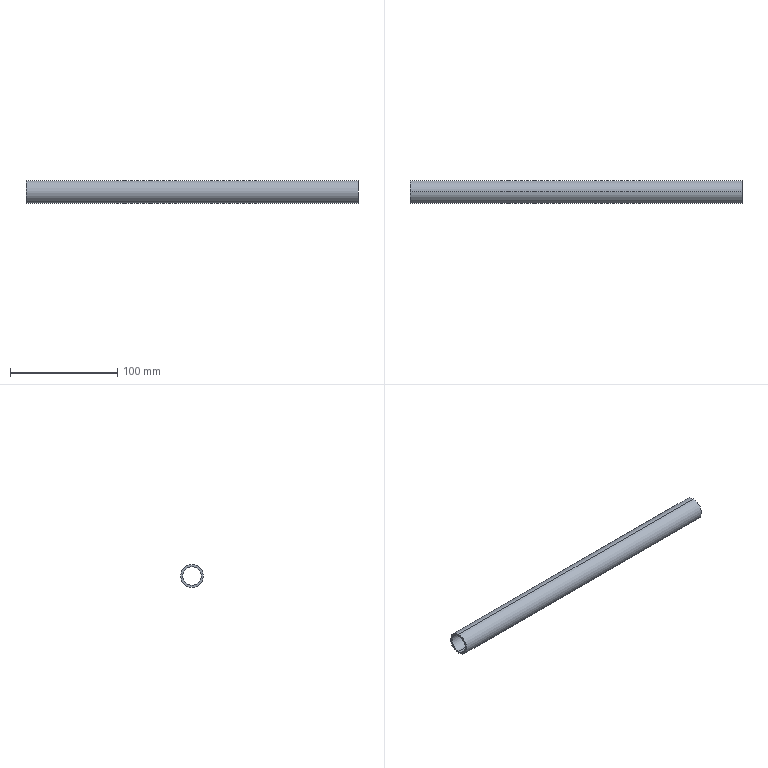Part | SolidWorks | features WeldMemberFeat 1, WeldmentFeature 1 | 1 solid | 6 faces | box 310 x 21.3 x 21.3 mm | volume 37592 mm3 | cylinder 4 | plane 2 | commonest cylinder face diameters 17.3 x2 21.3 x2
STEP:
#1=CARTESIAN_POINT('',(155.,0.,-10.65));
#2=VERTEX_POINT('',#1);
#3=CARTESIAN_POINT('',(155.,0.,10.65));
#4=VERTEX_POINT('',#3);
#5=CARTESIAN_POINT('',(155.,0.,0.));
#6=DIRECTION('',(1.,0.,0.));
#7=DIRECTION('',(0.,0.,-1.));
#8=AXIS2_PLACEMENT_3D('',#5,#6,#7);
#9=CIRCLE('',#8,10.65);
#10=EDGE_CURVE('',#2,#4,#9,.T.);
#11=ORIENTED_EDGE('',*,*,#10,.F.);
#12=CARTESIAN_POINT('',(-155.,0.,-10.65));
#13=VERTEX_POINT('',#12);
#14=CARTESIAN_POINT('',(155.,0.,-10.65));
#15=DIRECTION('',(-1.,0.,0.));
#16=VECTOR('',#15,1000.);
#17=LINE('',#14,#16);
#18=EDGE_CURVE('',#2,#13,#17,.T.);
#19=ORIENTED_EDGE('',*,*,#18,.T.);
#20=CARTESIAN_POINT('',(-155.,0.,10.65));
#21=VERTEX_POINT('',#20);
#22=CARTESIAN_POINT('',(-155.,0.,0.));
#23=DIRECTION('',(1.,0.,0.));
#24=DIRECTION('',(0.,0.,-1.));
#25=AXIS2_PLACEMENT_3D('',#22,#23,#24);
#26=CIRCLE('',#25,10.65);
#27=EDGE_CURVE('',#13,#21,#26,.T.);
#28=ORIENTED_EDGE('',*,*,#27,.T.);
#29=CARTESIAN_POINT('',(155.,0.,10.65));
#30=DIRECTION('',(-1.,0.,0.));
#31=VECTOR('',#30,1000.);
#32=LINE('',#29,#31);
#33=EDGE_CURVE('',#4,#21,#32,.T.);
#34=ORIENTED_EDGE('',*,*,#33,.F.);
#35=EDGE_LOOP('',(#11,#19,#28,#34));
#36=FACE_OUTER_BOUND('',#35,.T.);
#37=CARTESIAN_POINT('',(155.,0.,0.));
#38=DIRECTION('',(-1.,0.,0.));
#39=DIRECTION('',(0.,0.,1.));
#40=AXIS2_PLACEMENT_3D('',#37,#38,#39);
#41=CYLINDRICAL_SURFACE('',#40,10.65);
#42=ADVANCED_FACE('',(#36),#41,.T.);
#43=CARTESIAN_POINT('',(155.,0.,8.65));
#44=VERTEX_POINT('',#43);
#45=CARTESIAN_POINT('',(155.,0.,-8.65));
#46=VERTEX_POINT('',#45);
#47=CARTESIAN_POINT('',(155.,0.,0.));
#48=DIRECTION('',(1.,0.,0.));
#49=DIRECTION('',(0.,0.,-1.));
#50=AXIS2_PLACEMENT_3D('',#47,#48,#49);
#51=CIRCLE('',#50,8.65);
#52=EDGE_CURVE('',#44,#46,#51,.T.);
#53=ORIENTED_EDGE('',*,*,#52,.T.);
#54=CARTESIAN_POINT('',(-155.,0.,-8.65));
#55=VERTEX_POINT('',#54);
#56=CARTESIAN_POINT('',(155.,0.,-8.65));
#57=DIRECTION('',(-1.,0.,0.));
#58=VECTOR('',#57,1000.);
#59=LINE('',#56,#58);
#60=EDGE_CURVE('',#46,#55,#59,.T.);
#61=ORIENTED_EDGE('',*,*,#60,.T.);
#62=CARTESIAN_POINT('',(-155.,0.,8.65));
#63=VERTEX_POINT('',#62);
#64=CARTESIAN_POINT('',(-155.,0.,0.));
#65=DIRECTION('',(1.,0.,0.));
#66=DIRECTION('',(0.,0.,-1.));
#67=AXIS2_PLACEMENT_3D('',#64,#65,#66);
#68=CIRCLE('',#67,8.65);
#69=EDGE_CURVE('',#63,#55,#68,.T.);
#70=ORIENTED_EDGE('',*,*,#69,.F.);
#71=CARTESIAN_POINT('',(155.,0.,8.65));
#72=DIRECTION('',(-1.,0.,0.));
#73=VECTOR('',#72,1000.);
#74=LINE('',#71,#73);
#75=EDGE_CURVE('',#44,#63,#74,.T.);
#76=ORIENTED_EDGE('',*,*,#75,.F.);
#77=EDGE_LOOP('',(#53,#61,#70,#76));
#78=FACE_OUTER_BOUND('',#77,.T.);
#79=CARTESIAN_POINT('',(155.,0.,0.));
#80=DIRECTION('',(-1.,0.,0.));
#81=DIRECTION('',(0.,0.,1.));
#82=AXIS2_PLACEMENT_3D('',#79,#80,#81);
#83=CYLINDRICAL_SURFACE('',#82,8.65);
#84=ADVANCED_FACE('',(#78),#83,.F.);
#85=ORIENTED_EDGE('',*,*,#60,.F.);
#86=CARTESIAN_POINT('',(155.,0.,0.));
#87=DIRECTION('',(1.,0.,0.));
#88=DIRECTION('',(0.,0.,-1.));
#89=AXIS2_PLACEMENT_3D('',#86,#87,#88);
#90=CIRCLE('',#89,8.65);
#91=EDGE_CURVE('',#46,#44,#90,.T.);
#92=ORIENTED_EDGE('',*,*,#91,.T.);
#93=ORIENTED_EDGE('',*,*,#75,.T.);
#94=CARTESIAN_POINT('',(-155.,0.,0.));
#95=DIRECTION('',(1.,0.,0.));
#96=DIRECTION('',(0.,0.,-1.));
#97=AXIS2_PLACEMENT_3D('',#94,#95,#96);
#98=CIRCLE('',#97,8.65);
#99=EDGE_CURVE('',#55,#63,#98,.T.);
#100=ORIENTED_EDGE('',*,*,#99,.F.);
#101=EDGE_LOOP('',(#85,#92,#93,#100));
#102=FACE_OUTER_BOUND('',#101,.T.);
#103=CARTESIAN_POINT('',(155.,0.,0.));
#104=DIRECTION('',(-1.,0.,0.));
#105=DIRECTION('',(0.,0.,1.));
#106=AXIS2_PLACEMENT_3D('',#103,#104,#105);
#107=CYLINDRICAL_SURFACE('',#106,8.65);
#108=ADVANCED_FACE('',(#102),#107,.F.);
#109=ORIENTED_EDGE('',*,*,#18,.F.);
#110=CARTESIAN_POINT('',(155.,0.,0.));
#111=DIRECTION('',(1.,0.,0.));
#112=DIRECTION('',(0.,0.,-1.));
#113=AXIS2_PLACEMENT_3D('',#110,#111,#112);
#114=CIRCLE('',#113,10.65);
#115=EDGE_CURVE('',#4,#2,#114,.T.);
#116=ORIENTED_EDGE('',*,*,#115,.F.);
#117=ORIENTED_EDGE('',*,*,#33,.T.);
#118=CARTESIAN_POINT('',(-155.,0.,0.));
#119=DIRECTION('',(1.,0.,0.));
#120=DIRECTION('',(0.,0.,-1.));
#121=AXIS2_PLACEMENT_3D('',#118,#119,#120);
#122=CIRCLE('',#121,10.65);
#123=EDGE_CURVE('',#21,#13,#122,.T.);
#124=ORIENTED_EDGE('',*,*,#123,.T.);
#125=EDGE_LOOP('',(#109,#116,#117,#124));
#126=FACE_OUTER_BOUND('',#125,.T.);
#127=CARTESIAN_POINT('',(155.,0.,0.));
#128=DIRECTION('',(-1.,0.,0.));
#129=DIRECTION('',(0.,0.,1.));
#130=AXIS2_PLACEMENT_3D('',#127,#128,#129);
#131=CYLINDRICAL_SURFACE('',#130,10.65);
#132=ADVANCED_FACE('',(#126),#131,.T.);
#133=ORIENTED_EDGE('',*,*,#52,.F.);
#134=ORIENTED_EDGE('',*,*,#91,.F.);
#135=EDGE_LOOP('',(#133,#134));
#136=FACE_BOUND('',#135,.T.);
#137=ORIENTED_EDGE('',*,*,#115,.T.);
#138=ORIENTED_EDGE('',*,*,#10,.T.);
#139=EDGE_LOOP('',(#137,#138));
#140=FACE_OUTER_BOUND('',#139,.T.);
#141=CARTESIAN_POINT('',(155.,0.,0.));
#142=DIRECTION('',(1.,0.,0.));
#143=DIRECTION('',(0.,0.,-1.));
#144=AXIS2_PLACEMENT_3D('',#141,#142,#143);
#145=PLANE('',#144);
#146=ADVANCED_FACE('',(#136,#140),#145,.T.);
#147=ORIENTED_EDGE('',*,*,#69,.T.);
#148=ORIENTED_EDGE('',*,*,#99,.T.);
#149=EDGE_LOOP('',(#147,#148));
#150=FACE_BOUND('',#149,.T.);
#151=ORIENTED_EDGE('',*,*,#123,.F.);
#152=ORIENTED_EDGE('',*,*,#27,.F.);
#153=EDGE_LOOP('',(#151,#152));
#154=FACE_OUTER_BOUND('',#153,.T.);
#155=CARTESIAN_POINT('',(-155.,0.,0.));
#156=DIRECTION('',(1.,0.,0.));
#157=DIRECTION('',(0.,0.,-1.));
#158=AXIS2_PLACEMENT_3D('',#155,#156,#157);
#159=PLANE('',#158);
#160=ADVANCED_FACE('',(#150,#154),#159,.F.);
#161=CLOSED_SHELL('',(#42,#84,#108,#132,#146,#160));
#162=MANIFOLD_SOLID_BREP('',#161);
#163=CARTESIAN_POINT('',(0.,0.,0.));
#164=DIRECTION('',(0.,0.,1.));
#165=DIRECTION('',(1.,0.,0.));
#166=AXIS2_PLACEMENT_3D('',#163,#164,#165);
#167=(LENGTH_UNIT()NAMED_UNIT(*)SI_UNIT(.MILLI.,.METRE.));
#168=UNCERTAINTY_MEASURE_WITH_UNIT(LENGTH_MEASURE(0.00001),#167,'','');
#169=(NAMED_UNIT(*)PLANE_ANGLE_UNIT()SI_UNIT($,.RADIAN.));
#170=(NAMED_UNIT(*)SI_UNIT($,.STERADIAN.)SOLID_ANGLE_UNIT());
#171=(GEOMETRIC_REPRESENTATION_CONTEXT(3)GLOBAL_UNCERTAINTY_ASSIGNED_CONTEXT((#168))GLOBAL_UNIT_ASSIGNED_CONTEXT((#167,#169,#170))REPRESENTATION_CONTEXT('',''));
#172=ADVANCED_BREP_SHAPE_REPRESENTATION('',(#162,#166),#171);